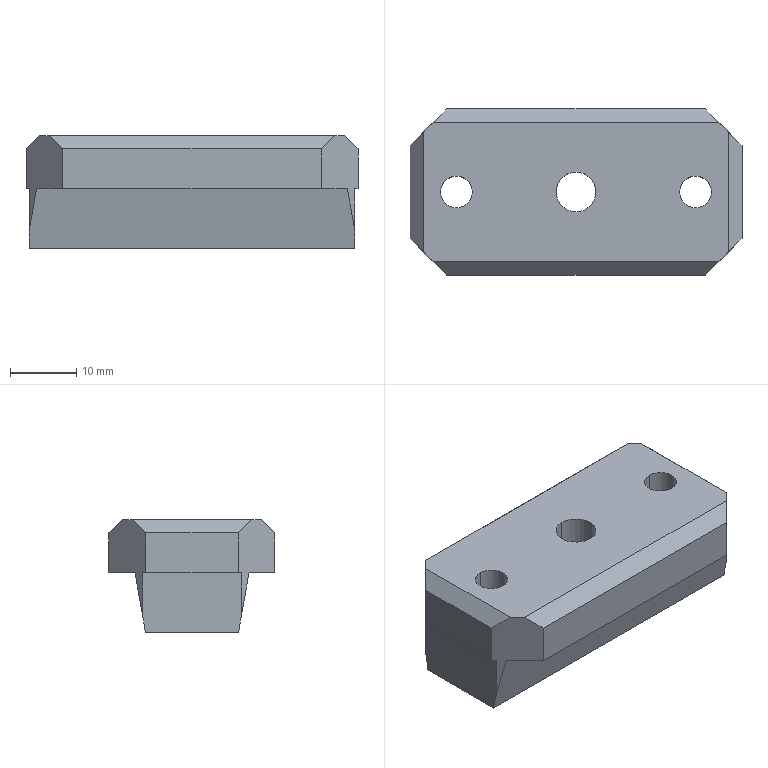Part | Creo | 1 solid | 31 faces | box 50 x 25 x 17 mm | volume 14766 mm3 | plane 23 | cylinder 8 | commonest cylinder face diameters 4.8 x4 6 x2 10 x2
STEP:
#1=CARTESIAN_POINT('',(19.5,-172.5,38.161));
#2=VERTEX_POINT('',#1);
#3=CARTESIAN_POINT('',(-19.5,-172.5,38.161));
#4=VERTEX_POINT('',#3);
#5=CARTESIAN_POINT('',(19.5,-172.5,38.161));
#6=DIRECTION('',(-1.,0.,0.));
#7=VECTOR('',#6,39.);
#8=LINE('',#5,#7);
#9=EDGE_CURVE('',#2,#4,#8,.T.);
#10=ORIENTED_EDGE('',*,*,#9,.F.);
#11=CARTESIAN_POINT('',(19.5,-172.5,44.161));
#12=VERTEX_POINT('',#11);
#13=CARTESIAN_POINT('',(19.5,-172.5,44.161));
#14=DIRECTION('',(0.,0.,-1.));
#15=VECTOR('',#14,6.);
#16=LINE('',#13,#15);
#17=EDGE_CURVE('',#12,#2,#16,.T.);
#18=ORIENTED_EDGE('',*,*,#17,.F.);
#19=CARTESIAN_POINT('',(-19.5,-172.5,44.161));
#20=VERTEX_POINT('',#19);
#21=CARTESIAN_POINT('',(-19.5,-172.5,44.161));
#22=DIRECTION('',(1.,0.,0.));
#23=VECTOR('',#22,39.);
#24=LINE('',#21,#23);
#25=EDGE_CURVE('',#20,#12,#24,.T.);
#26=ORIENTED_EDGE('',*,*,#25,.F.);
#27=CARTESIAN_POINT('',(-19.5,-172.5,38.161));
#28=DIRECTION('',(0.,0.,1.));
#29=VECTOR('',#28,6.);
#30=LINE('',#27,#29);
#31=EDGE_CURVE('',#4,#20,#30,.T.);
#32=ORIENTED_EDGE('',*,*,#31,.F.);
#33=EDGE_LOOP('',(#10,#18,#26,#32));
#34=FACE_OUTER_BOUND('',#33,.F.);
#35=CARTESIAN_POINT('',(25.,-172.5,38.161));
#36=DIRECTION('',(0.,-1.,0.));
#37=DIRECTION('',(0.,0.,1.));
#38=AXIS2_PLACEMENT_3D('',#35,#36,#37);
#39=PLANE('',#38);
#40=ADVANCED_FACE('',(#34),#39,.F.);
#41=CARTESIAN_POINT('',(-23.412,-176.412,38.161));
#42=VERTEX_POINT('',#41);
#43=CARTESIAN_POINT('',(-23.412,-176.412,38.161));
#44=DIRECTION('',(0.7071,0.7071,0.));
#45=VECTOR('',#44,5.532);
#46=LINE('',#43,#45);
#47=EDGE_CURVE('',#42,#4,#46,.T.);
#48=ORIENTED_EDGE('',*,*,#47,.F.);
#49=CARTESIAN_POINT('',(23.412,-176.412,38.161));
#50=VERTEX_POINT('',#49);
#51=CARTESIAN_POINT('',(23.412,-176.412,38.161));
#52=DIRECTION('',(-1.,0.,0.));
#53=VECTOR('',#52,46.823);
#54=LINE('',#51,#53);
#55=EDGE_CURVE('',#50,#42,#54,.T.);
#56=ORIENTED_EDGE('',*,*,#55,.F.);
#57=CARTESIAN_POINT('',(19.5,-172.5,38.161));
#58=DIRECTION('',(0.7071,-0.7071,0.));
#59=VECTOR('',#58,5.532);
#60=LINE('',#57,#59);
#61=EDGE_CURVE('',#2,#50,#60,.T.);
#62=ORIENTED_EDGE('',*,*,#61,.F.);
#63=ORIENTED_EDGE('',*,*,#9,.T.);
#64=EDGE_LOOP('',(#48,#56,#62,#63));
#65=FACE_OUTER_BOUND('',#64,.F.);
#66=CARTESIAN_POINT('',(-50.,-172.5,38.161));
#67=DIRECTION('',(0.,0.,-1.));
#68=DIRECTION('',(0.,-1.,0.));
#69=AXIS2_PLACEMENT_3D('',#66,#67,#68);
#70=PLANE('',#69);
#71=ADVANCED_FACE('',(#65),#70,.T.);
#72=CARTESIAN_POINT('',(-24.5,-177.5,38.161));
#73=VERTEX_POINT('',#72);
#74=CARTESIAN_POINT('',(-24.5,-177.5,31.989));
#75=VERTEX_POINT('',#74);
#76=CARTESIAN_POINT('',(-24.5,-177.5,38.161));
#77=DIRECTION('',(0.,0.,-1.));
#78=VECTOR('',#77,6.172);
#79=LINE('',#76,#78);
#80=EDGE_CURVE('',#73,#75,#79,.T.);
#81=ORIENTED_EDGE('',*,*,#80,.T.);
#82=CARTESIAN_POINT('',(-24.5,-177.5,31.989));
#83=DIRECTION('',(0.1711,0.1711,0.9703));
#84=VECTOR('',#83,6.361);
#85=LINE('',#82,#84);
#86=EDGE_CURVE('',#75,#42,#85,.T.);
#87=ORIENTED_EDGE('',*,*,#86,.T.);
#88=ORIENTED_EDGE('',*,*,#47,.T.);
#89=ORIENTED_EDGE('',*,*,#31,.T.);
#90=CARTESIAN_POINT('',(-21.5,-174.5,46.161));
#91=VERTEX_POINT('',#90);
#92=CARTESIAN_POINT('',(-19.5,-172.5,44.161));
#93=DIRECTION('',(-0.5774,-0.5774,0.5774));
#94=VECTOR('',#93,3.464);
#95=LINE('',#92,#94);
#96=EDGE_CURVE('',#20,#91,#95,.T.);
#97=ORIENTED_EDGE('',*,*,#96,.T.);
#98=CARTESIAN_POINT('',(-23.,-176.,46.161));
#99=VERTEX_POINT('',#98);
#100=CARTESIAN_POINT('',(-21.5,-174.5,46.161));
#101=DIRECTION('',(-0.7071,-0.7071,0.));
#102=VECTOR('',#101,2.121);
#103=LINE('',#100,#102);
#104=EDGE_CURVE('',#91,#99,#103,.T.);
#105=ORIENTED_EDGE('',*,*,#104,.T.);
#106=CARTESIAN_POINT('',(-25.,-178.,44.161));
#107=VERTEX_POINT('',#106);
#108=CARTESIAN_POINT('',(-23.,-176.,46.161));
#109=DIRECTION('',(-0.5774,-0.5774,-0.5774));
#110=VECTOR('',#109,3.464);
#111=LINE('',#108,#110);
#112=EDGE_CURVE('',#99,#107,#111,.T.);
#113=ORIENTED_EDGE('',*,*,#112,.T.);
#114=CARTESIAN_POINT('',(-25.,-178.,38.161));
#115=VERTEX_POINT('',#114);
#116=CARTESIAN_POINT('',(-25.,-178.,44.161));
#117=DIRECTION('',(0.,0.,-1.));
#118=VECTOR('',#117,6.);
#119=LINE('',#116,#118);
#120=EDGE_CURVE('',#107,#115,#119,.T.);
#121=ORIENTED_EDGE('',*,*,#120,.T.);
#122=CARTESIAN_POINT('',(-25.,-178.,38.161));
#123=DIRECTION('',(0.7071,0.7071,0.));
#124=VECTOR('',#123,0.7071);
#125=LINE('',#122,#124);
#126=EDGE_CURVE('',#115,#73,#125,.T.);
#127=ORIENTED_EDGE('',*,*,#126,.T.);
#128=EDGE_LOOP('',(#81,#87,#88,#89,#97,#105,#113,#121,#127));
#129=FACE_OUTER_BOUND('',#128,.F.);
#130=CARTESIAN_POINT('',(-19.5,-172.5,38.161));
#131=DIRECTION('',(-0.7071,0.7071,0.));
#132=DIRECTION('',(0.7071,0.7071,0.));
#133=AXIS2_PLACEMENT_3D('',#130,#131,#132);
#134=PLANE('',#133);
#135=ADVANCED_FACE('',(#129),#134,.T.);
#136=CARTESIAN_POINT('',(-24.5,-192.5,31.989));
#137=VERTEX_POINT('',#136);
#138=CARTESIAN_POINT('',(-24.5,-192.5,38.161));
#139=VERTEX_POINT('',#138);
#140=CARTESIAN_POINT('',(-24.5,-192.5,31.989));
#141=DIRECTION('',(0.,0.,1.));
#142=VECTOR('',#141,6.172);
#143=LINE('',#140,#142);
#144=EDGE_CURVE('',#137,#139,#143,.T.);
#145=ORIENTED_EDGE('',*,*,#144,.F.);
#146=CARTESIAN_POINT('',(-24.5,-192.001,29.161));
#147=VERTEX_POINT('',#146);
#148=CARTESIAN_POINT('',(-24.5,-192.001,29.161));
#149=DIRECTION('',(0.,-0.1736,0.9848));
#150=VECTOR('',#149,2.872);
#151=LINE('',#148,#150);
#152=EDGE_CURVE('',#147,#137,#151,.T.);
#153=ORIENTED_EDGE('',*,*,#152,.F.);
#154=CARTESIAN_POINT('',(-24.5,-177.999,29.161));
#155=VERTEX_POINT('',#154);
#156=CARTESIAN_POINT('',(-24.5,-192.001,29.161));
#157=DIRECTION('',(0.,1.,0.));
#158=VECTOR('',#157,14.003);
#159=LINE('',#156,#158);
#160=EDGE_CURVE('',#147,#155,#159,.T.);
#161=ORIENTED_EDGE('',*,*,#160,.T.);
#162=CARTESIAN_POINT('',(-24.5,-177.5,31.989));
#163=DIRECTION('',(0.,-0.1736,-0.9848));
#164=VECTOR('',#163,2.872);
#165=LINE('',#162,#164);
#166=EDGE_CURVE('',#75,#155,#165,.T.);
#167=ORIENTED_EDGE('',*,*,#166,.F.);
#168=ORIENTED_EDGE('',*,*,#80,.F.);
#169=CARTESIAN_POINT('',(-24.5,-177.5,38.161));
#170=DIRECTION('',(0.,-1.,0.));
#171=VECTOR('',#170,15.);
#172=LINE('',#169,#171);
#173=EDGE_CURVE('',#73,#139,#172,.T.);
#174=ORIENTED_EDGE('',*,*,#173,.T.);
#175=EDGE_LOOP('',(#145,#153,#161,#167,#168,#174));
#176=FACE_OUTER_BOUND('',#175,.F.);
#177=CARTESIAN_POINT('',(-24.5,-235.,38.161));
#178=DIRECTION('',(1.,0.,0.));
#179=DIRECTION('',(0.,-1.,0.));
#180=AXIS2_PLACEMENT_3D('',#177,#178,#179);
#181=PLANE('',#180);
#182=ADVANCED_FACE('',(#176),#181,.F.);
#183=ORIENTED_EDGE('',*,*,#144,.T.);
#184=CARTESIAN_POINT('',(-25.,-192.,38.161));
#185=VERTEX_POINT('',#184);
#186=CARTESIAN_POINT('',(-24.5,-192.5,38.161));
#187=DIRECTION('',(-0.7071,0.7071,0.));
#188=VECTOR('',#187,0.7071);
#189=LINE('',#186,#188);
#190=EDGE_CURVE('',#139,#185,#189,.T.);
#191=ORIENTED_EDGE('',*,*,#190,.T.);
#192=CARTESIAN_POINT('',(-25.,-192.,44.161));
#193=VERTEX_POINT('',#192);
#194=CARTESIAN_POINT('',(-25.,-192.,38.161));
#195=DIRECTION('',(0.,0.,1.));
#196=VECTOR('',#195,6.);
#197=LINE('',#194,#196);
#198=EDGE_CURVE('',#185,#193,#197,.T.);
#199=ORIENTED_EDGE('',*,*,#198,.T.);
#200=CARTESIAN_POINT('',(-23.,-194.,46.161));
#201=VERTEX_POINT('',#200);
#202=CARTESIAN_POINT('',(-25.,-192.,44.161));
#203=DIRECTION('',(0.5774,-0.5774,0.5774));
#204=VECTOR('',#203,3.464);
#205=LINE('',#202,#204);
#206=EDGE_CURVE('',#193,#201,#205,.T.);
#207=ORIENTED_EDGE('',*,*,#206,.T.);
#208=CARTESIAN_POINT('',(-21.5,-195.5,46.161));
#209=VERTEX_POINT('',#208);
#210=CARTESIAN_POINT('',(-23.,-194.,46.161));
#211=DIRECTION('',(0.7071,-0.7071,0.));
#212=VECTOR('',#211,2.121);
#213=LINE('',#210,#212);
#214=EDGE_CURVE('',#201,#209,#213,.T.);
#215=ORIENTED_EDGE('',*,*,#214,.T.);
#216=CARTESIAN_POINT('',(-19.5,-197.5,44.161));
#217=VERTEX_POINT('',#216);
#218=CARTESIAN_POINT('',(-21.5,-195.5,46.161));
#219=DIRECTION('',(0.5774,-0.5774,-0.5774));
#220=VECTOR('',#219,3.464);
#221=LINE('',#218,#220);
#222=EDGE_CURVE('',#209,#217,#221,.T.);
#223=ORIENTED_EDGE('',*,*,#222,.T.);
#224=CARTESIAN_POINT('',(-19.5,-197.5,38.161));
#225=VERTEX_POINT('',#224);
#226=CARTESIAN_POINT('',(-19.5,-197.5,44.161));
#227=DIRECTION('',(0.,0.,-1.));
#228=VECTOR('',#227,6.);
#229=LINE('',#226,#228);
#230=EDGE_CURVE('',#217,#225,#229,.T.);
#231=ORIENTED_EDGE('',*,*,#230,.T.);
#232=CARTESIAN_POINT('',(-23.412,-193.588,38.161));
#233=VERTEX_POINT('',#232);
#234=CARTESIAN_POINT('',(-19.5,-197.5,38.161));
#235=DIRECTION('',(-0.7071,0.7071,0.));
#236=VECTOR('',#235,5.532);
#237=LINE('',#234,#236);
#238=EDGE_CURVE('',#225,#233,#237,.T.);
#239=ORIENTED_EDGE('',*,*,#238,.T.);
#240=CARTESIAN_POINT('',(-23.412,-193.588,38.161));
#241=DIRECTION('',(-0.1711,0.1711,-0.9703));
#242=VECTOR('',#241,6.361);
#243=LINE('',#240,#242);
#244=EDGE_CURVE('',#233,#137,#243,.T.);
#245=ORIENTED_EDGE('',*,*,#244,.T.);
#246=EDGE_LOOP('',(#183,#191,#199,#207,#215,#223,#231,#239,#245));
#247=FACE_OUTER_BOUND('',#246,.F.);
#248=CARTESIAN_POINT('',(-19.5,-197.5,38.161));
#249=DIRECTION('',(-0.7071,-0.7071,0.));
#250=DIRECTION('',(-0.7071,0.7071,0.));
#251=AXIS2_PLACEMENT_3D('',#248,#249,#250);
#252=PLANE('',#251);
#253=ADVANCED_FACE('',(#247),#252,.T.);
#254=ORIENTED_EDGE('',*,*,#190,.F.);
#255=ORIENTED_EDGE('',*,*,#173,.F.);
#256=ORIENTED_EDGE('',*,*,#126,.F.);
#257=CARTESIAN_POINT('',(-25.,-178.,38.161));
#258=DIRECTION('',(0.,-1.,0.));
#259=VECTOR('',#258,14.);
#260=LINE('',#257,#259);
#261=EDGE_CURVE('',#115,#185,#260,.T.);
#262=ORIENTED_EDGE('',*,*,#261,.T.);
#263=EDGE_LOOP('',(#254,#255,#256,#262));
#264=FACE_OUTER_BOUND('',#263,.F.);
#265=CARTESIAN_POINT('',(-25.,-135.,38.161));
#266=DIRECTION('',(0.,0.,1.));
#267=DIRECTION('',(0.,1.,0.));
#268=AXIS2_PLACEMENT_3D('',#265,#266,#267);
#269=PLANE('',#268);
#270=ADVANCED_FACE('',(#264),#269,.F.);
#271=ORIENTED_EDGE('',*,*,#261,.F.);
#272=ORIENTED_EDGE('',*,*,#120,.F.);
#273=CARTESIAN_POINT('',(-25.,-192.,44.161));
#274=DIRECTION('',(0.,1.,0.));
#275=VECTOR('',#274,14.);
#276=LINE('',#273,#275);
#277=EDGE_CURVE('',#193,#107,#276,.T.);
#278=ORIENTED_EDGE('',*,*,#277,.F.);
#279=ORIENTED_EDGE('',*,*,#198,.F.);
#280=EDGE_LOOP('',(#271,#272,#278,#279));
#281=FACE_OUTER_BOUND('',#280,.F.);
#282=CARTESIAN_POINT('',(-25.,-197.5,46.161));
#283=DIRECTION('',(-1.,0.,0.));
#284=DIRECTION('',(0.,1.,0.));
#285=AXIS2_PLACEMENT_3D('',#282,#283,#284);
#286=PLANE('',#285);
#287=ADVANCED_FACE('',(#281),#286,.T.);
#288=CARTESIAN_POINT('',(-23.,-176.,46.161));
#289=DIRECTION('',(0.,-1.,0.));
#290=VECTOR('',#289,18.);
#291=LINE('',#288,#290);
#292=EDGE_CURVE('',#99,#201,#291,.T.);
#293=ORIENTED_EDGE('',*,*,#292,.T.);
#294=ORIENTED_EDGE('',*,*,#206,.F.);
#295=ORIENTED_EDGE('',*,*,#277,.T.);
#296=ORIENTED_EDGE('',*,*,#112,.F.);
#297=EDGE_LOOP('',(#293,#294,#295,#296));
#298=FACE_OUTER_BOUND('',#297,.F.);
#299=CARTESIAN_POINT('',(-23.,-197.5,46.161));
#300=DIRECTION('',(-0.7071,0.,0.7071));
#301=DIRECTION('',(-0.7071,0.,-0.7071));
#302=AXIS2_PLACEMENT_3D('',#299,#300,#301);
#303=PLANE('',#302);
#304=ADVANCED_FACE('',(#298),#303,.T.);
#305=CARTESIAN_POINT('',(21.5,-195.5,46.161));
#306=VERTEX_POINT('',#305);
#307=CARTESIAN_POINT('',(-21.5,-195.5,46.161));
#308=DIRECTION('',(1.,0.,0.));
#309=VECTOR('',#308,43.);
#310=LINE('',#307,#309);
#311=EDGE_CURVE('',#209,#306,#310,.T.);
#312=ORIENTED_EDGE('',*,*,#311,.F.);
#313=ORIENTED_EDGE('',*,*,#214,.F.);
#314=ORIENTED_EDGE('',*,*,#292,.F.);
#315=ORIENTED_EDGE('',*,*,#104,.F.);
#316=CARTESIAN_POINT('',(21.5,-174.5,46.161));
#317=VERTEX_POINT('',#316);
#318=CARTESIAN_POINT('',(21.5,-174.5,46.161));
#319=DIRECTION('',(-1.,0.,0.));
#320=VECTOR('',#319,43.);
#321=LINE('',#318,#320);
#322=EDGE_CURVE('',#317,#91,#321,.T.);
#323=ORIENTED_EDGE('',*,*,#322,.F.);
#324=CARTESIAN_POINT('',(23.,-176.,46.161));
#325=VERTEX_POINT('',#324);
#326=CARTESIAN_POINT('',(23.,-176.,46.161));
#327=DIRECTION('',(-0.7071,0.7071,0.));
#328=VECTOR('',#327,2.121);
#329=LINE('',#326,#328);
#330=EDGE_CURVE('',#325,#317,#329,.T.);
#331=ORIENTED_EDGE('',*,*,#330,.F.);
#332=CARTESIAN_POINT('',(23.,-194.,46.161));
#333=VERTEX_POINT('',#332);
#334=CARTESIAN_POINT('',(23.,-194.,46.161));
#335=DIRECTION('',(0.,1.,0.));
#336=VECTOR('',#335,18.);
#337=LINE('',#334,#336);
#338=EDGE_CURVE('',#333,#325,#337,.T.);
#339=ORIENTED_EDGE('',*,*,#338,.F.);
#340=CARTESIAN_POINT('',(21.5,-195.5,46.161));
#341=DIRECTION('',(0.7071,0.7071,0.));
#342=VECTOR('',#341,2.121);
#343=LINE('',#340,#342);
#344=EDGE_CURVE('',#306,#333,#343,.T.);
#345=ORIENTED_EDGE('',*,*,#344,.F.);
#346=EDGE_LOOP('',(#312,#313,#314,#315,#323,#331,#339,#345));
#347=FACE_OUTER_BOUND('',#346,.F.);
#348=CARTESIAN_POINT('',(18.,-187.4,46.161));
#349=VERTEX_POINT('',#348);
#350=CARTESIAN_POINT('',(18.,-182.6,46.161));
#351=VERTEX_POINT('',#350);
#352=CARTESIAN_POINT('',(18.,-185.,46.161));
#353=DIRECTION('',(0.,0.,-1.));
#354=DIRECTION('',(0.,-1.,0.));
#355=AXIS2_PLACEMENT_3D('',#352,#353,#354);
#356=CIRCLE('',#355,2.4);
#357=EDGE_CURVE('',#349,#351,#356,.T.);
#358=ORIENTED_EDGE('',*,*,#357,.F.);
#359=CARTESIAN_POINT('',(18.,-185.,46.161));
#360=DIRECTION('',(0.,0.,-1.));
#361=DIRECTION('',(0.,1.,0.));
#362=AXIS2_PLACEMENT_3D('',#359,#360,#361);
#363=CIRCLE('',#362,2.4);
#364=EDGE_CURVE('',#351,#349,#363,.T.);
#365=ORIENTED_EDGE('',*,*,#364,.F.);
#366=EDGE_LOOP('',(#358,#365));
#367=FACE_BOUND('',#366,.F.);
#368=CARTESIAN_POINT('',(0.,-188.,46.161));
#369=VERTEX_POINT('',#368);
#370=CARTESIAN_POINT('',(0.,-182.,46.161));
#371=VERTEX_POINT('',#370);
#372=CARTESIAN_POINT('',(0.,-185.,46.161));
#373=DIRECTION('',(0.,0.,-1.));
#374=DIRECTION('',(0.,-1.,0.));
#375=AXIS2_PLACEMENT_3D('',#372,#373,#374);
#376=CIRCLE('',#375,3.);
#377=EDGE_CURVE('',#369,#371,#376,.T.);
#378=ORIENTED_EDGE('',*,*,#377,.F.);
#379=CARTESIAN_POINT('',(0.,-185.,46.161));
#380=DIRECTION('',(0.,0.,-1.));
#381=DIRECTION('',(0.,1.,0.));
#382=AXIS2_PLACEMENT_3D('',#379,#380,#381);
#383=CIRCLE('',#382,3.);
#384=EDGE_CURVE('',#371,#369,#383,.T.);
#385=ORIENTED_EDGE('',*,*,#384,.F.);
#386=EDGE_LOOP('',(#378,#385));
#387=FACE_BOUND('',#386,.F.);
#388=CARTESIAN_POINT('',(-18.,-187.4,46.161));
#389=VERTEX_POINT('',#388);
#390=CARTESIAN_POINT('',(-18.,-182.6,46.161));
#391=VERTEX_POINT('',#390);
#392=CARTESIAN_POINT('',(-18.,-185.,46.161));
#393=DIRECTION('',(0.,0.,-1.));
#394=DIRECTION('',(0.,-1.,0.));
#395=AXIS2_PLACEMENT_3D('',#392,#393,#394);
#396=CIRCLE('',#395,2.4);
#397=EDGE_CURVE('',#389,#391,#396,.T.);
#398=ORIENTED_EDGE('',*,*,#397,.F.);
#399=CARTESIAN_POINT('',(-18.,-185.,46.161));
#400=DIRECTION('',(0.,0.,-1.));
#401=DIRECTION('',(0.,1.,0.));
#402=AXIS2_PLACEMENT_3D('',#399,#400,#401);
#403=CIRCLE('',#402,2.4);
#404=EDGE_CURVE('',#391,#389,#403,.T.);
#405=ORIENTED_EDGE('',*,*,#404,.F.);
#406=EDGE_LOOP('',(#398,#405));
#407=FACE_BOUND('',#406,.F.);
#408=CARTESIAN_POINT('',(25.,-197.5,46.161));
#409=DIRECTION('',(0.,0.,-1.));
#410=DIRECTION('',(0.,-1.,0.));
#411=AXIS2_PLACEMENT_3D('',#408,#409,#410);
#412=PLANE('',#411);
#413=ADVANCED_FACE('',(#347,#367,#387,#407),#412,.F.);
#414=CARTESIAN_POINT('',(-18.,-182.6,29.161));
#415=VERTEX_POINT('',#414);
#416=CARTESIAN_POINT('',(-18.,-187.4,29.161));
#417=VERTEX_POINT('',#416);
#418=CARTESIAN_POINT('',(-18.,-185.,29.161));
#419=DIRECTION('',(0.,0.,1.));
#420=DIRECTION('',(0.,1.,0.));
#421=AXIS2_PLACEMENT_3D('',#418,#419,#420);
#422=CIRCLE('',#421,2.4);
#423=EDGE_CURVE('',#415,#417,#422,.T.);
#424=ORIENTED_EDGE('',*,*,#423,.T.);
#425=CARTESIAN_POINT('',(-18.,-187.4,46.161));
#426=DIRECTION('',(0.,0.,-1.));
#427=VECTOR('',#426,17.);
#428=LINE('',#425,#427);
#429=EDGE_CURVE('',#389,#417,#428,.T.);
#430=ORIENTED_EDGE('',*,*,#429,.F.);
#431=ORIENTED_EDGE('',*,*,#397,.T.);
#432=CARTESIAN_POINT('',(-18.,-182.6,46.161));
#433=DIRECTION('',(0.,0.,-1.));
#434=VECTOR('',#433,17.);
#435=LINE('',#432,#434);
#436=EDGE_CURVE('',#391,#415,#435,.T.);
#437=ORIENTED_EDGE('',*,*,#436,.T.);
#438=EDGE_LOOP('',(#424,#430,#431,#437));
#439=FACE_OUTER_BOUND('',#438,.F.);
#440=CARTESIAN_POINT('',(-18.,-185.,46.161));
#441=DIRECTION('',(0.,0.,-1.));
#442=DIRECTION('',(0.,-1.,0.));
#443=AXIS2_PLACEMENT_3D('',#440,#441,#442);
#444=CYLINDRICAL_SURFACE('',#443,2.4);
#445=ADVANCED_FACE('',(#439),#444,.F.);
#446=CARTESIAN_POINT('',(24.5,-192.001,29.161));
#447=VERTEX_POINT('',#446);
#448=CARTESIAN_POINT('',(24.5,-192.001,29.161));
#449=DIRECTION('',(-1.,0.,0.));
#450=VECTOR('',#449,49.);
#451=LINE('',#448,#450);
#452=EDGE_CURVE('',#447,#147,#451,.T.);
#453=ORIENTED_EDGE('',*,*,#452,.F.);
#454=CARTESIAN_POINT('',(24.5,-177.999,29.161));
#455=VERTEX_POINT('',#454);
#456=CARTESIAN_POINT('',(24.5,-177.999,29.161));
#457=DIRECTION('',(0.,-1.,0.));
#458=VECTOR('',#457,14.003);
#459=LINE('',#456,#458);
#460=EDGE_CURVE('',#455,#447,#459,.T.);
#461=ORIENTED_EDGE('',*,*,#460,.F.);
#462=CARTESIAN_POINT('',(24.5,-177.999,29.161));
#463=DIRECTION('',(-1.,0.,0.));
#464=VECTOR('',#463,49.);
#465=LINE('',#462,#464);
#466=EDGE_CURVE('',#455,#155,#465,.T.);
#467=ORIENTED_EDGE('',*,*,#466,.T.);
#468=ORIENTED_EDGE('',*,*,#160,.F.);
#469=EDGE_LOOP('',(#453,#461,#467,#468));
#470=FACE_OUTER_BOUND('',#469,.F.);
#471=CARTESIAN_POINT('',(18.,-182.6,29.161));
#472=VERTEX_POINT('',#471);
#473=CARTESIAN_POINT('',(18.,-187.4,29.161));
#474=VERTEX_POINT('',#473);
#475=CARTESIAN_POINT('',(18.,-185.,29.161));
#476=DIRECTION('',(0.,0.,1.));
#477=DIRECTION('',(0.,1.,0.));
#478=AXIS2_PLACEMENT_3D('',#475,#476,#477);
#479=CIRCLE('',#478,2.4);
#480=EDGE_CURVE('',#472,#474,#479,.T.);
#481=ORIENTED_EDGE('',*,*,#480,.F.);
#482=CARTESIAN_POINT('',(18.,-185.,29.161));
#483=DIRECTION('',(0.,0.,1.));
#484=DIRECTION('',(0.,-1.,0.));
#485=AXIS2_PLACEMENT_3D('',#482,#483,#484);
#486=CIRCLE('',#485,2.4);
#487=EDGE_CURVE('',#474,#472,#486,.T.);
#488=ORIENTED_EDGE('',*,*,#487,.F.);
#489=EDGE_LOOP('',(#481,#488));
#490=FACE_BOUND('',#489,.F.);
#491=CARTESIAN_POINT('',(0.,-180.,29.161));
#492=VERTEX_POINT('',#491);
#493=CARTESIAN_POINT('',(0.,-190.,29.161));
#494=VERTEX_POINT('',#493);
#495=CARTESIAN_POINT('',(0.,-185.,29.161));
#496=DIRECTION('',(0.,0.,1.));
#497=DIRECTION('',(0.,1.,0.));
#498=AXIS2_PLACEMENT_3D('',#495,#496,#497);
#499=CIRCLE('',#498,5.);
#500=EDGE_CURVE('',#492,#494,#499,.T.);
#501=ORIENTED_EDGE('',*,*,#500,.F.);
#502=CARTESIAN_POINT('',(0.,-185.,29.161));
#503=DIRECTION('',(0.,0.,1.));
#504=DIRECTION('',(0.,-1.,0.));
#505=AXIS2_PLACEMENT_3D('',#502,#503,#504);
#506=CIRCLE('',#505,5.);
#507=EDGE_CURVE('',#494,#492,#506,.T.);
#508=ORIENTED_EDGE('',*,*,#507,.F.);
#509=EDGE_LOOP('',(#501,#508));
#510=FACE_BOUND('',#509,.F.);
#511=ORIENTED_EDGE('',*,*,#423,.F.);
#512=CARTESIAN_POINT('',(-18.,-185.,29.161));
#513=DIRECTION('',(0.,0.,1.));
#514=DIRECTION('',(0.,-1.,0.));
#515=AXIS2_PLACEMENT_3D('',#512,#513,#514);
#516=CIRCLE('',#515,2.4);
#517=EDGE_CURVE('',#417,#415,#516,.T.);
#518=ORIENTED_EDGE('',*,*,#517,.F.);
#519=EDGE_LOOP('',(#511,#518));
#520=FACE_BOUND('',#519,.F.);
#521=CARTESIAN_POINT('',(-50.,-192.001,29.161));
#522=DIRECTION('',(0.,0.,1.));
#523=DIRECTION('',(0.,1.,0.));
#524=AXIS2_PLACEMENT_3D('',#521,#522,#523);
#525=PLANE('',#524);
#526=ADVANCED_FACE('',(#470,#490,#510,#520),#525,.F.);
#527=CARTESIAN_POINT('',(0.,-190.,35.161));
#528=VERTEX_POINT('',#527);
#529=CARTESIAN_POINT('',(0.,-180.,35.161));
#530=VERTEX_POINT('',#529);
#531=CARTESIAN_POINT('',(0.,-185.,35.161));
#532=DIRECTION('',(0.,0.,-1.));
#533=DIRECTION('',(0.,-1.,0.));
#534=AXIS2_PLACEMENT_3D('',#531,#532,#533);
#535=CIRCLE('',#534,5.);
#536=EDGE_CURVE('',#528,#530,#535,.T.);
#537=ORIENTED_EDGE('',*,*,#536,.T.);
#538=CARTESIAN_POINT('',(0.,-180.,29.161));
#539=DIRECTION('',(0.,0.,1.));
#540=VECTOR('',#539,6.);
#541=LINE('',#538,#540);
#542=EDGE_CURVE('',#492,#530,#541,.T.);
#543=ORIENTED_EDGE('',*,*,#542,.F.);
#544=ORIENTED_EDGE('',*,*,#500,.T.);
#545=CARTESIAN_POINT('',(0.,-190.,29.161));
#546=DIRECTION('',(0.,0.,1.));
#547=VECTOR('',#546,6.);
#548=LINE('',#545,#547);
#549=EDGE_CURVE('',#494,#528,#548,.T.);
#550=ORIENTED_EDGE('',*,*,#549,.T.);
#551=EDGE_LOOP('',(#537,#543,#544,#550));
#552=FACE_OUTER_BOUND('',#551,.F.);
#553=CARTESIAN_POINT('',(0.,-185.,29.161));
#554=DIRECTION('',(0.,0.,1.));
#555=DIRECTION('',(0.,1.,0.));
#556=AXIS2_PLACEMENT_3D('',#553,#554,#555);
#557=CYLINDRICAL_SURFACE('',#556,5.);
#558=ADVANCED_FACE('',(#552),#557,.F.);
#559=CARTESIAN_POINT('',(0.,-185.,35.161));
#560=DIRECTION('',(0.,0.,-1.));
#561=DIRECTION('',(0.,1.,0.));
#562=AXIS2_PLACEMENT_3D('',#559,#560,#561);
#563=CIRCLE('',#562,5.);
#564=EDGE_CURVE('',#530,#528,#563,.T.);
#565=ORIENTED_EDGE('',*,*,#564,.F.);
#566=ORIENTED_EDGE('',*,*,#536,.F.);
#567=EDGE_LOOP('',(#565,#566));
#568=FACE_OUTER_BOUND('',#567,.F.);
#569=CARTESIAN_POINT('',(0.,-182.,35.161));
#570=VERTEX_POINT('',#569);
#571=CARTESIAN_POINT('',(0.,-188.,35.161));
#572=VERTEX_POINT('',#571);
#573=CARTESIAN_POINT('',(0.,-185.,35.161));
#574=DIRECTION('',(0.,0.,1.));
#575=DIRECTION('',(0.,1.,0.));
#576=AXIS2_PLACEMENT_3D('',#573,#574,#575);
#577=CIRCLE('',#576,3.);
#578=EDGE_CURVE('',#570,#572,#577,.T.);
#579=ORIENTED_EDGE('',*,*,#578,.F.);
#580=CARTESIAN_POINT('',(0.,-185.,35.161));
#581=DIRECTION('',(0.,0.,1.));
#582=DIRECTION('',(0.,-1.,0.));
#583=AXIS2_PLACEMENT_3D('',#580,#581,#582);
#584=CIRCLE('',#583,3.);
#585=EDGE_CURVE('',#572,#570,#584,.T.);
#586=ORIENTED_EDGE('',*,*,#585,.F.);
#587=EDGE_LOOP('',(#579,#586));
#588=FACE_BOUND('',#587,.F.);
#589=CARTESIAN_POINT('',(0.,-185.,35.161));
#590=DIRECTION('',(0.,0.,1.));
#591=DIRECTION('',(0.,1.,0.));
#592=AXIS2_PLACEMENT_3D('',#589,#590,#591);
#593=PLANE('',#592);
#594=ADVANCED_FACE('',(#568,#588),#593,.F.);
#595=ORIENTED_EDGE('',*,*,#564,.T.);
#596=ORIENTED_EDGE('',*,*,#549,.F.);
#597=ORIENTED_EDGE('',*,*,#507,.T.);
#598=ORIENTED_EDGE('',*,*,#542,.T.);
#599=EDGE_LOOP('',(#595,#596,#597,#598));
#600=FACE_OUTER_BOUND('',#599,.F.);
#601=CARTESIAN_POINT('',(0.,-185.,29.161));
#602=DIRECTION('',(0.,0.,1.));
#603=DIRECTION('',(0.,1.,0.));
#604=AXIS2_PLACEMENT_3D('',#601,#602,#603);
#605=CYLINDRICAL_SURFACE('',#604,5.);
#606=ADVANCED_FACE('',(#600),#605,.F.);
#607=ORIENTED_EDGE('',*,*,#578,.T.);
#608=CARTESIAN_POINT('',(0.,-188.,46.161));
#609=DIRECTION('',(0.,0.,-1.));
#610=VECTOR('',#609,11.);
#611=LINE('',#608,#610);
#612=EDGE_CURVE('',#369,#572,#611,.T.);
#613=ORIENTED_EDGE('',*,*,#612,.F.);
#614=ORIENTED_EDGE('',*,*,#377,.T.);
#615=CARTESIAN_POINT('',(0.,-182.,46.161));
#616=DIRECTION('',(0.,0.,-1.));
#617=VECTOR('',#616,11.);
#618=LINE('',#615,#617);
#619=EDGE_CURVE('',#371,#570,#618,.T.);
#620=ORIENTED_EDGE('',*,*,#619,.T.);
#621=EDGE_LOOP('',(#607,#613,#614,#620));
#622=FACE_OUTER_BOUND('',#621,.F.);
#623=CARTESIAN_POINT('',(0.,-185.,46.161));
#624=DIRECTION('',(0.,0.,-1.));
#625=DIRECTION('',(0.,-1.,0.));
#626=AXIS2_PLACEMENT_3D('',#623,#624,#625);
#627=CYLINDRICAL_SURFACE('',#626,3.);
#628=ADVANCED_FACE('',(#622),#627,.F.);
#629=ORIENTED_EDGE('',*,*,#585,.T.);
#630=ORIENTED_EDGE('',*,*,#619,.F.);
#631=ORIENTED_EDGE('',*,*,#384,.T.);
#632=ORIENTED_EDGE('',*,*,#612,.T.);
#633=EDGE_LOOP('',(#629,#630,#631,#632));
#634=FACE_OUTER_BOUND('',#633,.F.);
#635=CARTESIAN_POINT('',(0.,-185.,46.161));
#636=DIRECTION('',(0.,0.,-1.));
#637=DIRECTION('',(0.,-1.,0.));
#638=AXIS2_PLACEMENT_3D('',#635,#636,#637);
#639=CYLINDRICAL_SURFACE('',#638,3.);
#640=ADVANCED_FACE('',(#634),#639,.F.);
#641=ORIENTED_EDGE('',*,*,#480,.T.);
#642=CARTESIAN_POINT('',(18.,-187.4,46.161));
#643=DIRECTION('',(0.,0.,-1.));
#644=VECTOR('',#643,17.);
#645=LINE('',#642,#644);
#646=EDGE_CURVE('',#349,#474,#645,.T.);
#647=ORIENTED_EDGE('',*,*,#646,.F.);
#648=ORIENTED_EDGE('',*,*,#357,.T.);
#649=CARTESIAN_POINT('',(18.,-182.6,46.161));
#650=DIRECTION('',(0.,0.,-1.));
#651=VECTOR('',#650,17.);
#652=LINE('',#649,#651);
#653=EDGE_CURVE('',#351,#472,#652,.T.);
#654=ORIENTED_EDGE('',*,*,#653,.T.);
#655=EDGE_LOOP('',(#641,#647,#648,#654));
#656=FACE_OUTER_BOUND('',#655,.F.);
#657=CARTESIAN_POINT('',(18.,-185.,46.161));
#658=DIRECTION('',(0.,0.,-1.));
#659=DIRECTION('',(0.,-1.,0.));
#660=AXIS2_PLACEMENT_3D('',#657,#658,#659);
#661=CYLINDRICAL_SURFACE('',#660,2.4);
#662=ADVANCED_FACE('',(#656),#661,.F.);
#663=ORIENTED_EDGE('',*,*,#487,.T.);
#664=ORIENTED_EDGE('',*,*,#653,.F.);
#665=ORIENTED_EDGE('',*,*,#364,.T.);
#666=ORIENTED_EDGE('',*,*,#646,.T.);
#667=EDGE_LOOP('',(#663,#664,#665,#666));
#668=FACE_OUTER_BOUND('',#667,.F.);
#669=CARTESIAN_POINT('',(18.,-185.,46.161));
#670=DIRECTION('',(0.,0.,-1.));
#671=DIRECTION('',(0.,-1.,0.));
#672=AXIS2_PLACEMENT_3D('',#669,#670,#671);
#673=CYLINDRICAL_SURFACE('',#672,2.4);
#674=ADVANCED_FACE('',(#668),#673,.F.);
#675=CARTESIAN_POINT('',(24.5,-192.5,31.989));
#676=VERTEX_POINT('',#675);
#677=CARTESIAN_POINT('',(23.412,-193.588,38.161));
#678=VERTEX_POINT('',#677);
#679=CARTESIAN_POINT('',(24.5,-192.5,31.989));
#680=DIRECTION('',(-0.1711,-0.1711,0.9703));
#681=VECTOR('',#680,6.361);
#682=LINE('',#679,#681);
#683=EDGE_CURVE('',#676,#678,#682,.T.);
#684=ORIENTED_EDGE('',*,*,#683,.F.);
#685=CARTESIAN_POINT('',(24.5,-192.5,31.989));
#686=DIRECTION('',(0.,0.1736,-0.9848));
#687=VECTOR('',#686,2.872);
#688=LINE('',#685,#687);
#689=EDGE_CURVE('',#676,#447,#688,.T.);
#690=ORIENTED_EDGE('',*,*,#689,.T.);
#691=ORIENTED_EDGE('',*,*,#452,.T.);
#692=ORIENTED_EDGE('',*,*,#152,.T.);
#693=ORIENTED_EDGE('',*,*,#244,.F.);
#694=CARTESIAN_POINT('',(23.412,-193.588,38.161));
#695=DIRECTION('',(-1.,0.,0.));
#696=VECTOR('',#695,46.823);
#697=LINE('',#694,#696);
#698=EDGE_CURVE('',#678,#233,#697,.T.);
#699=ORIENTED_EDGE('',*,*,#698,.F.);
#700=EDGE_LOOP('',(#684,#690,#691,#692,#693,#699));
#701=FACE_OUTER_BOUND('',#700,.F.);
#702=CARTESIAN_POINT('',(-50.,-193.588,38.161));
#703=DIRECTION('',(0.,0.9848,0.1736));
#704=DIRECTION('',(0.,0.1736,-0.9848));
#705=AXIS2_PLACEMENT_3D('',#702,#703,#704);
#706=PLANE('',#705);
#707=ADVANCED_FACE('',(#701),#706,.F.);
#708=CARTESIAN_POINT('',(24.5,-192.5,38.161));
#709=VERTEX_POINT('',#708);
#710=CARTESIAN_POINT('',(24.5,-192.5,38.161));
#711=DIRECTION('',(0.,0.,-1.));
#712=VECTOR('',#711,6.172);
#713=LINE('',#710,#712);
#714=EDGE_CURVE('',#709,#676,#713,.T.);
#715=ORIENTED_EDGE('',*,*,#714,.T.);
#716=ORIENTED_EDGE('',*,*,#683,.T.);
#717=CARTESIAN_POINT('',(19.5,-197.5,38.161));
#718=VERTEX_POINT('',#717);
#719=CARTESIAN_POINT('',(23.412,-193.588,38.161));
#720=DIRECTION('',(-0.7071,-0.7071,0.));
#721=VECTOR('',#720,5.532);
#722=LINE('',#719,#721);
#723=EDGE_CURVE('',#678,#718,#722,.T.);
#724=ORIENTED_EDGE('',*,*,#723,.T.);
#725=CARTESIAN_POINT('',(19.5,-197.5,44.161));
#726=VERTEX_POINT('',#725);
#727=CARTESIAN_POINT('',(19.5,-197.5,38.161));
#728=DIRECTION('',(0.,0.,1.));
#729=VECTOR('',#728,6.);
#730=LINE('',#727,#729);
#731=EDGE_CURVE('',#718,#726,#730,.T.);
#732=ORIENTED_EDGE('',*,*,#731,.T.);
#733=CARTESIAN_POINT('',(19.5,-197.5,44.161));
#734=DIRECTION('',(0.5774,0.5774,0.5774));
#735=VECTOR('',#734,3.464);
#736=LINE('',#733,#735);
#737=EDGE_CURVE('',#726,#306,#736,.T.);
#738=ORIENTED_EDGE('',*,*,#737,.T.);
#739=ORIENTED_EDGE('',*,*,#344,.T.);
#740=CARTESIAN_POINT('',(25.,-192.,44.161));
#741=VERTEX_POINT('',#740);
#742=CARTESIAN_POINT('',(23.,-194.,46.161));
#743=DIRECTION('',(0.5774,0.5774,-0.5774));
#744=VECTOR('',#743,3.464);
#745=LINE('',#742,#744);
#746=EDGE_CURVE('',#333,#741,#745,.T.);
#747=ORIENTED_EDGE('',*,*,#746,.T.);
#748=CARTESIAN_POINT('',(25.,-192.,38.161));
#749=VERTEX_POINT('',#748);
#750=CARTESIAN_POINT('',(25.,-192.,44.161));
#751=DIRECTION('',(0.,0.,-1.));
#752=VECTOR('',#751,6.);
#753=LINE('',#750,#752);
#754=EDGE_CURVE('',#741,#749,#753,.T.);
#755=ORIENTED_EDGE('',*,*,#754,.T.);
#756=CARTESIAN_POINT('',(25.,-192.,38.161));
#757=DIRECTION('',(-0.7071,-0.7071,0.));
#758=VECTOR('',#757,0.7071);
#759=LINE('',#756,#758);
#760=EDGE_CURVE('',#749,#709,#759,.T.);
#761=ORIENTED_EDGE('',*,*,#760,.T.);
#762=EDGE_LOOP('',(#715,#716,#724,#732,#738,#739,#747,#755,#761));
#763=FACE_OUTER_BOUND('',#762,.F.);
#764=CARTESIAN_POINT('',(25.,-192.,46.161));
#765=DIRECTION('',(-0.7071,0.7071,0.));
#766=DIRECTION('',(0.7071,0.7071,0.));
#767=AXIS2_PLACEMENT_3D('',#764,#765,#766);
#768=PLANE('',#767);
#769=ADVANCED_FACE('',(#763),#768,.F.);
#770=ORIENTED_EDGE('',*,*,#714,.F.);
#771=CARTESIAN_POINT('',(24.5,-177.5,38.161));
#772=VERTEX_POINT('',#771);
#773=CARTESIAN_POINT('',(24.5,-177.5,38.161));
#774=DIRECTION('',(0.,-1.,0.));
#775=VECTOR('',#774,15.);
#776=LINE('',#773,#775);
#777=EDGE_CURVE('',#772,#709,#776,.T.);
#778=ORIENTED_EDGE('',*,*,#777,.F.);
#779=CARTESIAN_POINT('',(24.5,-177.5,31.989));
#780=VERTEX_POINT('',#779);
#781=CARTESIAN_POINT('',(24.5,-177.5,31.989));
#782=DIRECTION('',(0.,0.,1.));
#783=VECTOR('',#782,6.172);
#784=LINE('',#781,#783);
#785=EDGE_CURVE('',#780,#772,#784,.T.);
#786=ORIENTED_EDGE('',*,*,#785,.F.);
#787=CARTESIAN_POINT('',(24.5,-177.999,29.161));
#788=DIRECTION('',(0.,0.1736,0.9848));
#789=VECTOR('',#788,2.872);
#790=LINE('',#787,#789);
#791=EDGE_CURVE('',#455,#780,#790,.T.);
#792=ORIENTED_EDGE('',*,*,#791,.F.);
#793=ORIENTED_EDGE('',*,*,#460,.T.);
#794=ORIENTED_EDGE('',*,*,#689,.F.);
#795=EDGE_LOOP('',(#770,#778,#786,#792,#793,#794));
#796=FACE_OUTER_BOUND('',#795,.F.);
#797=CARTESIAN_POINT('',(24.5,-235.,38.161));
#798=DIRECTION('',(-1.,0.,0.));
#799=DIRECTION('',(0.,-1.,0.));
#800=AXIS2_PLACEMENT_3D('',#797,#798,#799);
#801=PLANE('',#800);
#802=ADVANCED_FACE('',(#796),#801,.F.);
#803=CARTESIAN_POINT('',(25.,-178.,38.161));
#804=VERTEX_POINT('',#803);
#805=CARTESIAN_POINT('',(24.5,-177.5,38.161));
#806=DIRECTION('',(0.7071,-0.7071,0.));
#807=VECTOR('',#806,0.7071);
#808=LINE('',#805,#807);
#809=EDGE_CURVE('',#772,#804,#808,.T.);
#810=ORIENTED_EDGE('',*,*,#809,.F.);
#811=ORIENTED_EDGE('',*,*,#777,.T.);
#812=ORIENTED_EDGE('',*,*,#760,.F.);
#813=CARTESIAN_POINT('',(25.,-178.,38.161));
#814=DIRECTION('',(0.,-1.,0.));
#815=VECTOR('',#814,14.);
#816=LINE('',#813,#815);
#817=EDGE_CURVE('',#804,#749,#816,.T.);
#818=ORIENTED_EDGE('',*,*,#817,.F.);
#819=EDGE_LOOP('',(#810,#811,#812,#818));
#820=FACE_OUTER_BOUND('',#819,.F.);
#821=CARTESIAN_POINT('',(25.,-135.,38.161));
#822=DIRECTION('',(0.,0.,1.));
#823=DIRECTION('',(0.,1.,0.));
#824=AXIS2_PLACEMENT_3D('',#821,#822,#823);
#825=PLANE('',#824);
#826=ADVANCED_FACE('',(#820),#825,.F.);
#827=ORIENTED_EDGE('',*,*,#785,.T.);
#828=ORIENTED_EDGE('',*,*,#809,.T.);
#829=CARTESIAN_POINT('',(25.,-178.,44.161));
#830=VERTEX_POINT('',#829);
#831=CARTESIAN_POINT('',(25.,-178.,38.161));
#832=DIRECTION('',(0.,0.,1.));
#833=VECTOR('',#832,6.);
#834=LINE('',#831,#833);
#835=EDGE_CURVE('',#804,#830,#834,.T.);
#836=ORIENTED_EDGE('',*,*,#835,.T.);
#837=CARTESIAN_POINT('',(25.,-178.,44.161));
#838=DIRECTION('',(-0.5774,0.5774,0.5774));
#839=VECTOR('',#838,3.464);
#840=LINE('',#837,#839);
#841=EDGE_CURVE('',#830,#325,#840,.T.);
#842=ORIENTED_EDGE('',*,*,#841,.T.);
#843=ORIENTED_EDGE('',*,*,#330,.T.);
#844=CARTESIAN_POINT('',(21.5,-174.5,46.161));
#845=DIRECTION('',(-0.5774,0.5774,-0.5774));
#846=VECTOR('',#845,3.464);
#847=LINE('',#844,#846);
#848=EDGE_CURVE('',#317,#12,#847,.T.);
#849=ORIENTED_EDGE('',*,*,#848,.T.);
#850=ORIENTED_EDGE('',*,*,#17,.T.);
#851=ORIENTED_EDGE('',*,*,#61,.T.);
#852=CARTESIAN_POINT('',(23.412,-176.412,38.161));
#853=DIRECTION('',(0.1711,-0.1711,-0.9703));
#854=VECTOR('',#853,6.361);
#855=LINE('',#852,#854);
#856=EDGE_CURVE('',#50,#780,#855,.T.);
#857=ORIENTED_EDGE('',*,*,#856,.T.);
#858=EDGE_LOOP('',(#827,#828,#836,#842,#843,#849,#850,#851,#857));
#859=FACE_OUTER_BOUND('',#858,.F.);
#860=CARTESIAN_POINT('',(25.,-178.,46.161));
#861=DIRECTION('',(-0.7071,-0.7071,0.));
#862=DIRECTION('',(-0.7071,0.7071,0.));
#863=AXIS2_PLACEMENT_3D('',#860,#861,#862);
#864=PLANE('',#863);
#865=ADVANCED_FACE('',(#859),#864,.F.);
#866=ORIENTED_EDGE('',*,*,#835,.F.);
#867=ORIENTED_EDGE('',*,*,#817,.T.);
#868=ORIENTED_EDGE('',*,*,#754,.F.);
#869=CARTESIAN_POINT('',(25.,-178.,44.161));
#870=DIRECTION('',(0.,-1.,0.));
#871=VECTOR('',#870,14.);
#872=LINE('',#869,#871);
#873=EDGE_CURVE('',#830,#741,#872,.T.);
#874=ORIENTED_EDGE('',*,*,#873,.F.);
#875=EDGE_LOOP('',(#866,#867,#868,#874));
#876=FACE_OUTER_BOUND('',#875,.F.);
#877=CARTESIAN_POINT('',(25.,-197.5,46.161));
#878=DIRECTION('',(-1.,0.,0.));
#879=DIRECTION('',(0.,1.,0.));
#880=AXIS2_PLACEMENT_3D('',#877,#878,#879);
#881=PLANE('',#880);
#882=ADVANCED_FACE('',(#876),#881,.F.);
#883=ORIENTED_EDGE('',*,*,#338,.T.);
#884=ORIENTED_EDGE('',*,*,#841,.F.);
#885=ORIENTED_EDGE('',*,*,#873,.T.);
#886=ORIENTED_EDGE('',*,*,#746,.F.);
#887=EDGE_LOOP('',(#883,#884,#885,#886));
#888=FACE_OUTER_BOUND('',#887,.F.);
#889=CARTESIAN_POINT('',(25.,-197.5,44.161));
#890=DIRECTION('',(-0.7071,0.,-0.7071));
#891=DIRECTION('',(0.7071,0.,-0.7071));
#892=AXIS2_PLACEMENT_3D('',#889,#890,#891);
#893=PLANE('',#892);
#894=ADVANCED_FACE('',(#888),#893,.F.);
#895=ORIENTED_EDGE('',*,*,#322,.T.);
#896=ORIENTED_EDGE('',*,*,#96,.F.);
#897=ORIENTED_EDGE('',*,*,#25,.T.);
#898=ORIENTED_EDGE('',*,*,#848,.F.);
#899=EDGE_LOOP('',(#895,#896,#897,#898));
#900=FACE_OUTER_BOUND('',#899,.F.);
#901=CARTESIAN_POINT('',(25.,-172.5,44.161));
#902=DIRECTION('',(0.,-0.7071,-0.7071));
#903=DIRECTION('',(0.,-0.7071,0.7071));
#904=AXIS2_PLACEMENT_3D('',#901,#902,#903);
#905=PLANE('',#904);
#906=ADVANCED_FACE('',(#900),#905,.F.);
#907=ORIENTED_EDGE('',*,*,#466,.F.);
#908=ORIENTED_EDGE('',*,*,#791,.T.);
#909=ORIENTED_EDGE('',*,*,#856,.F.);
#910=ORIENTED_EDGE('',*,*,#55,.T.);
#911=ORIENTED_EDGE('',*,*,#86,.F.);
#912=ORIENTED_EDGE('',*,*,#166,.T.);
#913=EDGE_LOOP('',(#907,#908,#909,#910,#911,#912));
#914=FACE_OUTER_BOUND('',#913,.F.);
#915=CARTESIAN_POINT('',(-50.,-177.999,29.161));
#916=DIRECTION('',(0.,-0.9848,0.1736));
#917=DIRECTION('',(0.,0.1736,0.9848));
#918=AXIS2_PLACEMENT_3D('',#915,#916,#917);
#919=PLANE('',#918);
#920=ADVANCED_FACE('',(#914),#919,.F.);
#921=ORIENTED_EDGE('',*,*,#698,.T.);
#922=ORIENTED_EDGE('',*,*,#238,.F.);
#923=CARTESIAN_POINT('',(19.5,-197.5,38.161));
#924=DIRECTION('',(-1.,0.,0.));
#925=VECTOR('',#924,39.);
#926=LINE('',#923,#925);
#927=EDGE_CURVE('',#718,#225,#926,.T.);
#928=ORIENTED_EDGE('',*,*,#927,.F.);
#929=ORIENTED_EDGE('',*,*,#723,.F.);
#930=EDGE_LOOP('',(#921,#922,#928,#929));
#931=FACE_OUTER_BOUND('',#930,.F.);
#932=CARTESIAN_POINT('',(-50.,-197.5,38.161));
#933=DIRECTION('',(0.,0.,1.));
#934=DIRECTION('',(0.,1.,0.));
#935=AXIS2_PLACEMENT_3D('',#932,#933,#934);
#936=PLANE('',#935);
#937=ADVANCED_FACE('',(#931),#936,.F.);
#938=ORIENTED_EDGE('',*,*,#731,.F.);
#939=ORIENTED_EDGE('',*,*,#927,.T.);
#940=ORIENTED_EDGE('',*,*,#230,.F.);
#941=CARTESIAN_POINT('',(19.5,-197.5,44.161));
#942=DIRECTION('',(-1.,0.,0.));
#943=VECTOR('',#942,39.);
#944=LINE('',#941,#943);
#945=EDGE_CURVE('',#726,#217,#944,.T.);
#946=ORIENTED_EDGE('',*,*,#945,.F.);
#947=EDGE_LOOP('',(#938,#939,#940,#946));
#948=FACE_OUTER_BOUND('',#947,.F.);
#949=CARTESIAN_POINT('',(25.,-197.5,38.161));
#950=DIRECTION('',(0.,1.,0.));
#951=DIRECTION('',(0.,0.,-1.));
#952=AXIS2_PLACEMENT_3D('',#949,#950,#951);
#953=PLANE('',#952);
#954=ADVANCED_FACE('',(#948),#953,.F.);
#955=ORIENTED_EDGE('',*,*,#945,.T.);
#956=ORIENTED_EDGE('',*,*,#222,.F.);
#957=ORIENTED_EDGE('',*,*,#311,.T.);
#958=ORIENTED_EDGE('',*,*,#737,.F.);
#959=EDGE_LOOP('',(#955,#956,#957,#958));
#960=FACE_OUTER_BOUND('',#959,.F.);
#961=CARTESIAN_POINT('',(25.,-195.5,46.161));
#962=DIRECTION('',(0.,0.7071,-0.7071));
#963=DIRECTION('',(0.,-0.7071,-0.7071));
#964=AXIS2_PLACEMENT_3D('',#961,#962,#963);
#965=PLANE('',#964);
#966=ADVANCED_FACE('',(#960),#965,.F.);
#967=ORIENTED_EDGE('',*,*,#517,.T.);
#968=ORIENTED_EDGE('',*,*,#436,.F.);
#969=ORIENTED_EDGE('',*,*,#404,.T.);
#970=ORIENTED_EDGE('',*,*,#429,.T.);
#971=EDGE_LOOP('',(#967,#968,#969,#970));
#972=FACE_OUTER_BOUND('',#971,.F.);
#973=CARTESIAN_POINT('',(-18.,-185.,46.161));
#974=DIRECTION('',(0.,0.,-1.));
#975=DIRECTION('',(0.,-1.,0.));
#976=AXIS2_PLACEMENT_3D('',#973,#974,#975);
#977=CYLINDRICAL_SURFACE('',#976,2.4);
#978=ADVANCED_FACE('',(#972),#977,.F.);
#979=CLOSED_SHELL('',(#40,#71,#135,#182,#253,#270,#287,#304,#413,#445,#526,#558,#594,#606,#628,#640,#662,#674,#707,#769,#802,#826,#865,#882,#894,#906,#920,#937,#954,#966,#978));
#980=MANIFOLD_SOLID_BREP('',#979);
#981=(LENGTH_UNIT()NAMED_UNIT(*)SI_UNIT(.MILLI.,.METRE.));
#982=UNCERTAINTY_MEASURE_WITH_UNIT(LENGTH_MEASURE(0.005843),#981,'','');
#983=(NAMED_UNIT(*)PLANE_ANGLE_UNIT()SI_UNIT($,.RADIAN.));
#984=PLANE_ANGLE_MEASURE_WITH_UNIT(PLANE_ANGLE_MEASURE(0.01745),#983);
#985=(CONVERSION_BASED_UNIT('DEGREE',#984)NAMED_UNIT(*)PLANE_ANGLE_UNIT());
#986=(NAMED_UNIT(*)SI_UNIT($,.STERADIAN.)SOLID_ANGLE_UNIT());
#987=(GEOMETRIC_REPRESENTATION_CONTEXT(3)GLOBAL_UNCERTAINTY_ASSIGNED_CONTEXT((#982))GLOBAL_UNIT_ASSIGNED_CONTEXT((#981,#985,#986))REPRESENTATION_CONTEXT('',''));
#988=ADVANCED_BREP_SHAPE_REPRESENTATION('',(#980),#987);